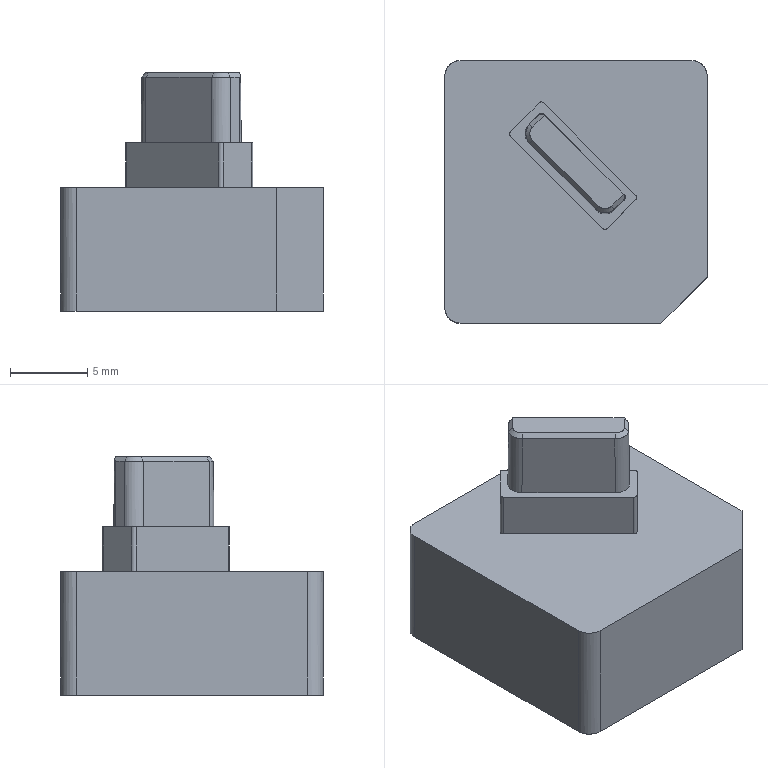NC program | PowerMill | posted with a generic post | part box 17 x 17 x 15.424 mm
Lines 2608 to 3246 of 24748:
N2705 M6
N2706 S8500 M03
N2707 G00 G90 X0.0 Y0.0
N2708 G43 Z11.804 H3
N2709
N2710 G05 P10000 R8
N2711 X-8.1622 Y14.5705
N2712 Z-3.7092
N2713 G01 Z-4.9092 F360.0
N2714 X-5.2505 Y10.1719 F600.0
N2715 X-4.7795 Y9.7047
N2716 G03 X-5.672 Y9.1307 I3.0048 J-5.6526
N2717 G01 X-5.9261 Y8.9205
N2718 X-6.1665 Y8.6947
N2719 X-6.7532 Y8.1079
N2720 X-6.943 Y7.9079
N2721 G03 X-7.4693 Y7.2473 I6.5097 J-5.7258
N2722 G01 X-7.6194 Y7.014
N2723 X-7.7808 Y6.7353
N2724 X-7.9298 Y6.4498
N2725 X-8.4896 Y7.0052
N2726 G00 Z5.8713
N2727 G01 X-8.3234 Y5.386 F10000.0
N2728 G00 Z-4.8092
N2729 G01 X-8.1838 Y5.8632 Z-4.8179 F360.0
N2730 X-8.0732 Y6.142 Z-4.8231
N2731 X-7.861 Y6.5856 Z-4.8317
N2732 X-7.6194 Y7.014 Z-4.8403
N2733 X-7.4693 Y7.2473 Z-4.8451
N2734 X-7.2142 Y7.584 Z-4.8525
N2735 X-6.943 Y7.9079 Z-4.8599
N2736 X-6.7692 Y8.0911 Z-4.8643
N2737 X-6.7532 Y8.1079 Z-4.8647
N2738 X-6.1665 Y8.6947 Z-4.8792
N2739 X-5.9261 Y8.9205 Z-4.8849
N2740 X-5.672 Y9.1307 Z-4.8907
N2741 X-5.2377 Y9.4362 Z-4.8999
N2742 X-4.7795 Y9.7047 Z-4.9092
N2743 X-4.408 Y9.8803 F600.0
N2744 X-4.0874 Y10.0038
N2745 X-3.7594 Y10.1061
N2746 G02 X-2.9536 Y10.2721 I1.8952 J-7.163
N2747 G01 X-2.5982 Y10.3085
N2748 X-2.2411 Y10.3207
N2749 X-1.884 Y10.3085
N2750 X-1.5285 Y10.2721
N2751 X-1.0566 Y10.1868
N2752 X-0.7227 Y10.1061
N2753 G02 X-0.0742 Y9.8803 I-1.5958 J-5.6266
N2754 G01 X0.2376 Y9.736
N2755 G02 X0.8297 Y9.388 I-2.6446 J-5.1761
N2756 G01 X1.1898 Y9.1307
N2757 X1.4429 Y8.9192
N2758 X1.6843 Y8.6947
N2759 X6.8169 Y3.5621
N2760 X7.0418 Y3.3209
N2761 X7.2529 Y3.0676
N2762 G02 X7.6939 Y2.4171 I-5.8869 J-4.466
N2763 G01 X7.8582 Y2.1154
N2764 X8.0025 Y1.8036
N2765 G02 X8.2429 Y1.0948 I-4.9188 J-2.0636
N2766 G01 X8.3338 Y0.7014
N2767 X8.3943 Y0.3493
N2768 G02 X8.4429 Y-0.3633 I-6.2851 J-0.7865
N2769 G01 X8.4307 Y-0.7204
N2770 X8.3943 Y-1.0759
N2771 X8.3338 Y-1.428
N2772 X8.2257 Y-1.8902
N2773 X8.126 Y-2.2096
N2774 G02 X7.8582 Y-2.842 I-5.4983 J1.9554
N2775 G01 X7.6939 Y-3.1437
N2776 X7.5102 Y-3.434
N2777 G02 X7.0427 Y-4.0483 I-5.0394 J3.3504
N2778 G01 X6.8169 Y-4.2887
N2779 X6.3459 Y-4.7598
N2780 G02 X5.5221 Y-5.4769 I-4.7037 J4.5714
N2781 G01 X5.3696 Y-5.5915
N2782 X5.0503 Y-5.797
N2783 G02 X4.2642 Y-6.1955 I-4.3291 J7.5645
N2784 G01 X3.9854 Y-6.3061
N2785 X3.7008 Y-6.4006
N2786 G02 X2.6002 Y-6.6355 I-2.1014 J7.1496
N2787 G01 X2.2932 Y-6.6626
N2788 X1.8786 Y-6.672
N2789 X1.464 Y-6.6626
N2790 X1.1571 Y-6.6355
N2791 X0.8523 Y-6.5904
N2792 G02 X-0.2282 Y-6.306 I1.3299 J7.2474
N2793 G01 X-0.507 Y-6.1955
N2794 G02 X-1.6123 Y-5.5915 I2.7732 J6.3884
N2795 G01 X-1.9159 Y-5.3635
N2796 G02 X-2.4729 Y-4.8755 I3.9536 J5.0749
N2797 G01 X-6.7532 Y-0.5952
N2798 G02 X-7.2412 Y-0.0381 I4.6108 J4.5318
N2799 G01 X-7.4692 Y0.2654
N2800 X-7.6747 Y0.5847
N2801 G02 X-8.0732 Y1.3708 I7.6482 J4.3716
N2802 G02 X-8.3564 Y2.2238 I5.0677 J2.1558
N2803 G02 X-8.5133 Y3.0348 I6.3457 J1.648
N2804 G01 X-8.5404 Y3.3418
N2805 G02 X-8.5133 Y4.4779 I7.4238 J0.3914
N2806 G02 X-8.1838 Y5.8632 I6.9185 J-0.9134
N2807 G01 X-8.0732 Y6.142
N2808 G02 X-7.6194 Y7.014 I6.7125 J-2.9395
N2809 G01 X-7.4693 Y7.2473
N2810 G02 X-6.943 Y7.9079 I7.036 J-5.0652
N2811 G01 X-6.7532 Y8.1079
N2812 X-6.1665 Y8.6947
N2813 X-5.9261 Y8.9205
N2814 X-5.672 Y9.1307
N2815 G02 X-4.7795 Y9.7047 I3.8973 J-5.0786
N2816 G00 Z4.0043
N2817 G01 X11.9477 Y-5.849 F10000.0
N2818 G00 Z0.8043
N2819 G01 Z-0.3957 F360.0
N2820 X7.4899 Y-3.0288 F600.0
N2821 X-4.7276 Y9.4739
N2822 X-4.9227 Y9.3603
N2823 X-5.3702 Y9.0347
N2824 X-5.4753 Y8.947
N2825 X-5.8176 Y8.6272
N2826 X-6.7123 Y7.7236
N2827 X-6.8167 Y7.605
N2828 X-7.1706 Y7.1572
N2829 X-7.4577 Y6.7094
N2830 X-7.5609 Y6.5138
N2831 X4.4533 Y-5.7809
N2832 G00 Z11.804
N2833 G05 P0
N2834 (---------------)
N2835 ( END TOOLPATH : 粗公基准台01-平坦面平行-D10 )
N2836 (---------------)
N2837 ( START TOOLPATH : 粗公基准台01-基准面偏置-D10 )
N2838 (---------------)
N2839 G00 X0.0 Y0.0 Z9.8043
N2840 G05 P10000 R8
N2841 X-2.368 Y19.035
N2842 Z-6.42
N2843 G01 Z-7.62 F360.0
N2844 X-2.3679 Y13.76 F600.0
N2845 X-2.3306 Y11.0677
N2846 G02 X-1.5285 Y11.0212 I0.0777 J-5.5932
N2847 G01 X-1.0969 Y10.9442
N2848 X-0.763 Y10.8635
N2849 X-0.435 Y10.7612
N2850 G02 X0.1974 Y10.4935 I-1.9637 J-5.5178
N2851 G01 X0.4991 Y10.3291
N2852 G02 X1.1182 Y9.9094 I-3.4177 J-5.708
N2853 G01 X1.3715 Y9.6983
N2854 X1.6127 Y9.4735
N2855 X7.5957 Y3.4904
N2856 X7.8214 Y3.25
N2857 G02 X8.6157 Y2.0751 I-4.4126 J-3.8388
N2858 G01 X8.7599 Y1.7633
N2859 X8.8835 Y1.4428
N2860 X8.9858 Y1.1148
N2861 X9.0664 Y0.7809
N2862 G02 X9.1798 Y-0.0062 I-5.9029 J-1.2522
N2863 G01 X9.192 Y-0.3633
N2864 X9.1798 Y-0.7204
N2865 X9.1434 Y-1.0758
N2866 X9.0659 Y-1.5095
N2867 X8.9858 Y-1.8414
N2868 X8.8835 Y-2.1694
N2869 X8.7599 Y-2.4899
N2870 X8.6157 Y-2.8017
N2871 X8.4513 Y-3.1034
N2872 X8.2255 Y-3.4557
N2873 X8.0317 Y-3.7225
N2874 X7.8215 Y-3.9766
N2875 X7.5957 Y-4.217
N2876 X5.7323 Y-6.0804
N2877 X5.4912 Y-6.3053
N2878 X5.2378 Y-6.5163
N2879 G02 X4.317 Y-7.1003 I-3.6863 J4.7942
N2880 G01 X4.0052 Y-7.2446
N2881 X3.6847 Y-7.3681
N2882 X3.3567 Y-7.4704
N2883 G02 X2.2357 Y-7.6645 I-1.6096 J5.9637
N2884 G02 X1.0756 Y-7.6125 I-0.3458 J5.2547
N2885 G01 X0.7345 Y-7.5511
N2886 G02 X-0.5822 Y-7.0882 I1.0963 J5.2223
N2887 G01 X-0.8615 Y-6.936
N2888 G02 X-1.4806 Y-6.5164 I3.4923 J5.8183
N2889 G01 X-1.7339 Y-6.3052
N2890 X-1.9751 Y-6.0804
N2891 X-3.5935 Y-4.462
N2892 X-6.991 Y-7.8595
N2893 G02 X-7.8827 Y-8.7514 I-0.4459 J-0.4459
N2894 G01 X-8.7516 Y-7.8829
N2895 G02 X-8.7517 Y-6.9908 I0.4459 J0.4461
N2896 G02 X-7.8596 I0.446 J-0.446
N2897 G01 X-6.991 Y-7.8595
N2898 X-3.5935 Y-4.462
N2899 X-7.9582 Y-0.0973
N2900 X-8.1829 Y0.144
N2901 X-8.3941 Y0.3971
N2902 X-8.6301 Y0.7259
N2903 X-8.8138 Y1.0163
N2904 X-8.9781 Y1.3179
N2905 X-9.1224 Y1.6298
N2906 X-9.2459 Y1.9503
N2907 G02 X-9.4453 Y2.6917 I5.5688 J1.8955
N2908 G01 X-9.5058 Y3.0438
N2909 X-9.5423 Y3.3993
N2910 X-9.5544 Y3.7564
N2911 X-9.5423 Y4.1135
N2912 X-9.5058 Y4.4689
N2913 X-9.4289 Y4.9005
N2914 X-9.3482 Y5.2345
N2915 X-9.2459 Y5.5624
N2916 G02 X-8.9781 Y6.1948 I5.5451 J-1.9752
N2917 G02 X-8.5484 Y6.9033 I4.9388 J-2.5112
N2918 G01 X-8.3941 Y7.1156
N2919 X-8.1839 Y7.3697
N2920 X-7.9582 Y7.6101
N2921 X-6.0948 Y9.4735
N2922 G02 X-5.2715 Y10.1454 I3.9028 J-3.9416
N2923 G01 X-4.9812 Y10.3291
N2924 X-4.6795 Y10.4935
N2925 X-4.3677 Y10.6377
N2926 X-4.0467 Y10.76
N2927 X-3.7192 Y10.8636
N2928 G02 X-2.9536 Y11.0211 I1.7771 J-6.6944
N2929 G01 X-2.5982 Y11.0576
N2930 X-2.3306 Y11.0677
N2931 X-2.3679 Y13.76
N2932 G00 Z9.8043
N2933 G05 P0
N2934 (---------------)
N2935 ( END TOOLPATH : 粗公基准台01-基准面偏置-D10 )
N2936 (---------------)
N2937 ( START TOOLPATH : 粗公基准台01-外形侧光-D10 )
N2938 (---------------)
N2939 G00 X0.0 Y0.0 Z10.804
N2940 G05 P10000 R8
N2941 X7.47 Y-4.439
N2942 Z-6.39
N2943 G01 Z-7.59 F360.0
N2944 G03 X6.4095 Y-4.8787 I0.0005 J-1.5 F600.0
N2945 G01 X5.4224 Y-5.8664
N2946 G02 X-1.6666 Y-5.865 I-3.5438 J3.6493
N2947 G01 X-4.6693 Y-2.8626
N2948 X-7.6732 Y0.141
N2949 G02 X-7.6721 Y7.373 I3.5784 J3.6154
N2950 G01 X-6.8152 Y8.2298
N2951 X-5.8221 Y9.2228
N2952 G02 X1.3419 Y9.221 I3.5811 J-3.6118
N2953 G01 X7.2798 Y3.2831
N2954 G02 X7.4142 Y-3.8733 I-3.5486 J-3.6461
N2955 G01 X6.4095 Y-4.8787
N2956 G03 X5.9705 Y-5.9395 I1.061 J-1.0603
N2957 G01 X7.4133 Y-4.3825
N2958 G03 X6.3528 Y-4.8222 I0.0005 J-1.5
N2959 G01 X5.3673 Y-5.8084
N2960 G02 X-1.6101 I-3.4887 J3.5911
N2961 G01 X-4.6128 Y-2.806
N2962 X-7.6155 Y0.1964
N2963 G02 Y7.3164 I3.5206 J3.56
N2964 G01 X-6.7586 Y8.1732
N2965 X-5.7675 Y9.1644
N2966 G02 X1.2853 I3.5264 J-3.5534
N2967 G01 X7.3573 Y3.0905
N2968 G02 Y-3.8171 I-3.6245 J-3.4538
N2969 G01 X6.3528 Y-4.8222
N2970 G03 X5.9138 Y-5.883 I1.061 J-1.0603
N2971 G00 Z10.804
N2972 G05 P0
N2973 (---------------)
N2974 ( END TOOLPATH : 粗公基准台01-外形侧光-D10 )
N2975 (---------------)
N2976 ( START TOOLPATH : 粗公基准台01-基准台侧光-D10 )
N2977 (---------------)
N2978 G00 X0.0 Y0.0 Z9.8043
N2979 G05 P10000 R8
N2980 X13.4843 Y-14.7706
N2981 Z-14.32
N2982 G01 Z-15.52 F360.0
N2983 G03 X9.9488 Y-11.2351 I-1.7677 J1.7677 F600.0
N2984 G01 X9.0587 Y-12.1252
N2985 X9.0582 Y-12.1257
N2986 X9.0577 Y-12.1262
N2987 X8.9953 Y-12.1864
N2988 X8.9933 Y-12.1883
N2989 X8.9913 Y-12.19
N2990 X8.5443 Y-12.5666
N2991 X8.5408 Y-12.5694
N2992 X8.5371 Y-12.572
N2993 X8.0901 Y-12.87
N2994 X8.0872 Y-12.8719
N2995 X8.0842 Y-12.8736
N2996 X7.7935 Y-13.0328
N2997 X7.7918 Y-13.0337
N2998 X7.79 Y-13.0346
N2999 X7.6336 Y-13.1102
N3000 X7.6312 Y-13.1114
N3001 X7.6288 Y-13.1124
N3002 X7.1818 Y-13.2935
N3003 X7.1783 Y-13.2948
N3004 X7.1746 Y-13.296
N3005 X6.7277 Y-13.4293
N3006 X6.7248 Y-13.4301
N3007 X6.722 Y-13.4308
N3008 X6.4639 Y-13.4877
N3009 X6.4621 Y-13.4881
N3010 X6.4603 Y-13.4884
N3011 X6.2714 Y-13.5211
N3012 X6.2689 Y-13.5215
N3013 X6.2664 Y-13.5218
N3014 X5.8194 Y-13.5699
N3015 X5.816 Y-13.5702
N3016 X5.8125 Y-13.5704
N3017 X5.3656 Y-13.58
N3018 X5.3647
N3019 X5.3638
N3020 X-7.5988 Y-13.5791
N3021 X-7.6011 Y-13.579
N3022 X-7.6033 Y-13.5789
N3023 X-8.0503 Y-13.5532
N3024 X-8.053 Y-13.553
N3025 X-8.0557 Y-13.5527
N3026 X-8.5027 Y-13.4965
N3027 X-8.5059 Y-13.496
N3028 X-8.5091 Y-13.4954
N3029 X-8.9561 Y-13.4017
N3030 X-8.9589 Y-13.4011
N3031 X-8.9617 Y-13.4003
N3032 X-9.4087 Y-13.2723
N3033 X-9.4118 Y-13.2713
N3034 X-9.4148 Y-13.2703
N3035 X-9.8618 Y-13.1025
N3036 X-9.8649 Y-13.1013
N3037 X-9.8679 Y-13.0999
N3038 X-10.3149 Y-12.8887
N3039 X-10.3178 Y-12.8872
N3040 X-10.3208 Y-12.8856
N3041 X-10.7677 Y-12.6268
N3042 X-10.7708 Y-12.6249
N3043 X-10.7738 Y-12.6229
N3044 X-11.2208 Y-12.3073
N3045 X-11.2238 Y-12.3051
N3046 X-11.2266 Y-12.3027
N3047 X-11.6736 Y-11.9205
N3048 X-11.676 Y-11.9184
N3049 X-11.6782 Y-11.9163
N3050 X-11.9163 Y-11.6782
N3051 X-11.9184 Y-11.676
N3052 X-11.9205 Y-11.6736
N3053 X-12.3027 Y-11.2266
N3054 X-12.3049 Y-11.224
N3055 X-12.307 Y-11.2213
N3056 X-12.5806 Y-10.8396
N3057 X-12.5827 Y-10.8365
N3058 X-12.5846 Y-10.8334
N3059 X-12.8853 Y-10.3212
N3060 X-12.8871 Y-10.318
N3061 X-12.8887 Y-10.3149
N3062 X-13.0999 Y-9.8679
N3063 X-13.1013 Y-9.8649
N3064 X-13.1025 Y-9.8618
N3065 X-13.2703 Y-9.4148
N3066 X-13.2713 Y-9.4118
N3067 X-13.2723 Y-9.4087
N3068 X-13.4003 Y-8.9617
N3069 X-13.4011 Y-8.9591
N3070 X-13.4017 Y-8.9564
N3071 X-13.4878 Y-8.5527
N3072 X-13.4884 Y-8.5495
N3073 X-13.4889 Y-8.5463
N3074 X-13.5527 Y-8.0561
N3075 X-13.553 Y-8.0532
N3076 X-13.5532 Y-8.0503
N3077 X-13.5789 Y-7.6033
N3078 X-13.579 Y-7.6011
N3079 X-13.5791 Y-7.5988
N3080 Y7.5988
N3081 X-13.579 Y7.6011
N3082 X-13.5789 Y7.6033
N3083 X-13.5532 Y8.0503
N3084 X-13.553 Y8.053
N3085 X-13.5527 Y8.0557
N3086 X-13.4965 Y8.5027
N3087 X-13.496 Y8.5059
N3088 X-13.4954 Y8.5091
N3089 X-13.4017 Y8.9561
N3090 X-13.4011 Y8.9589
N3091 X-13.4003 Y8.9617
N3092 X-13.2723 Y9.4087
N3093 X-13.2713 Y9.4118
N3094 X-13.2703 Y9.4148
N3095 X-13.1025 Y9.8618
N3096 X-13.1013 Y9.8649
N3097 X-13.0999 Y9.8679
N3098 X-12.8887 Y10.3149
N3099 X-12.8872 Y10.3178
N3100 X-12.8856 Y10.3208
N3101 X-12.6268 Y10.7677
N3102 X-12.6249 Y10.7708
N3103 X-12.6229 Y10.7738
N3104 X-12.3073 Y11.2208
N3105 X-12.3051 Y11.2238
N3106 X-12.3027 Y11.2266
N3107 X-11.9205 Y11.6736
N3108 X-11.9184 Y11.676
N3109 X-11.9163 Y11.6782
N3110 X-11.6782 Y11.9163
N3111 X-11.676 Y11.9184
N3112 X-11.6736 Y11.9205
N3113 X-11.2266 Y12.3027
N3114 X-11.224 Y12.3049
N3115 X-11.2213 Y12.307
N3116 X-10.8396 Y12.5806
N3117 X-10.8365 Y12.5827
N3118 X-10.8334 Y12.5846
N3119 X-10.3212 Y12.8853
N3120 X-10.318 Y12.8871
N3121 X-10.3149 Y12.8887
N3122 X-9.8679 Y13.0999
N3123 X-9.8649 Y13.1013
N3124 X-9.8618 Y13.1025
N3125 X-9.4148 Y13.2703
N3126 X-9.4118 Y13.2713
N3127 X-9.4087 Y13.2723
N3128 X-8.9617 Y13.4003
N3129 X-8.9591 Y13.4011
N3130 X-8.9564 Y13.4017
N3131 X-8.5527 Y13.4878
N3132 X-8.5495 Y13.4884
N3133 X-8.5463 Y13.4889
N3134 X-8.0561 Y13.5527
N3135 X-8.0532 Y13.553
N3136 X-8.0503 Y13.5532
N3137 X-7.6033 Y13.5789
N3138 X-7.6011 Y13.579
N3139 X-7.5988 Y13.5791
N3140 X0.0
N3141 X7.5988
N3142 X7.601 Y13.579
N3143 X7.6033 Y13.5789
N3144 X8.0503 Y13.5533
N3145 X8.053 Y13.5531
N3146 X8.0557 Y13.5528
N3147 X8.5027 Y13.4965
N3148 X8.5059 Y13.496
N3149 X8.5091 Y13.4954
N3150 X8.9561 Y13.4017
N3151 X8.9589 Y13.4011
N3152 X8.9617 Y13.4003
N3153 X9.4087 Y13.2723
N3154 X9.4118 Y13.2713
N3155 X9.4148 Y13.2703
N3156 X9.8618 Y13.1025
N3157 X9.8649 Y13.1013
N3158 X9.8679 Y13.0999
N3159 X10.3149 Y12.8887
N3160 X10.3178 Y12.8872
N3161 X10.3208 Y12.8856
N3162 X10.7677 Y12.6268
N3163 X10.7708 Y12.6249
N3164 X10.7738 Y12.6229
N3165 X11.2208 Y12.3073
N3166 X11.2238 Y12.3051
N3167 X11.2266 Y12.3027
N3168 X11.6736 Y11.9205
N3169 X11.676 Y11.9184
N3170 X11.6782 Y11.9163
N3171 X11.9163 Y11.6782
N3172 X11.9184 Y11.676
N3173 X11.9205 Y11.6736
N3174 X12.3027 Y11.2266
N3175 X12.3049 Y11.224
N3176 X12.307 Y11.2213
N3177 X12.5806 Y10.8396
N3178 X12.5827 Y10.8365
N3179 X12.5846 Y10.8334
N3180 X12.8853 Y10.3212
N3181 X12.8871 Y10.318
N3182 X12.8887 Y10.3149
N3183 X13.0999 Y9.8679
N3184 X13.1013 Y9.8649
N3185 X13.1025 Y9.8618
N3186 X13.2703 Y9.4148
N3187 X13.2713 Y9.4118
N3188 X13.2723 Y9.4087
N3189 X13.4003 Y8.9617
N3190 X13.401 Y8.9591
N3191 X13.4016 Y8.9564
N3192 X13.4878 Y8.5527
N3193 X13.4884 Y8.5495
N3194 X13.4889 Y8.5463
N3195 X13.5527 Y8.0561
N3196 X13.553 Y8.0532
N3197 X13.5532 Y8.0503
N3198 X13.5789 Y7.6033
N3199 X13.579 Y7.6011
N3200 X13.5791 Y7.5988
N3201 X13.58 Y-5.3638
N3202 Y-5.3647
N3203 Y-5.3656
N3204 X13.5704 Y-5.8125
N3205 X13.5702 Y-5.816
N3206 X13.5699 Y-5.8194
N3207 X13.5218 Y-6.2664
N3208 X13.5215 Y-6.2689
N3209 X13.5211 Y-6.2715
N3210 X13.4884 Y-6.4603
N3211 X13.4881 Y-6.4621
N3212 X13.4877 Y-6.4639
N3213 X13.4308 Y-6.722
N3214 X13.4301 Y-6.7248
N3215 X13.4293 Y-6.7277
N3216 X13.296 Y-7.1746
N3217 X13.2948 Y-7.1783
N3218 X13.2935 Y-7.1818
N3219 X13.1124 Y-7.6288
N3220 X13.1114 Y-7.6312
N3221 X13.1102 Y-7.6336
N3222 X13.0346 Y-7.79
N3223 X13.0337 Y-7.7918
N3224 X13.0328 Y-7.7935
N3225 X12.8736 Y-8.0842
N3226 X12.8719 Y-8.0871
N3227 X12.8701 Y-8.09
N3228 X12.5822 Y-8.5234
N3229 X12.5797 Y-8.527
N3230 X12.5769 Y-8.5305
N3231 X12.1901 Y-8.9912
N3232 X12.1883 Y-8.9932
N3233 X12.1864 Y-8.9953
N3234 X12.1262 Y-9.0577
N3235 X12.1257 Y-9.0582
N3236 X12.1252 Y-9.0587
N3237 X9.9488 Y-11.2351
N3238 G03 X13.4843 Y-14.7706 I1.7678 J-1.7678
N3239 G01 X13.433 Y-14.7089
N3240 G03 X9.8974 Y-11.1733 I-1.7678 J1.7678
N3241 G01 X9.0022 Y-12.0686
N3242 X8.9397 Y-12.1289
N3243 X8.4927 Y-12.5055
N3244 X8.0457 Y-12.8034
N3245 X7.7551 Y-12.9626
N3246 X7.5988 Y-13.0382
N3247 X7.1518 Y-13.2193
N3248 X6.7048 Y-13.3527
N3249 X6.4467 Y-13.4096
N3250 X6.2578 Y-13.4422
N3251 X5.8108 Y-13.4904
N3252 X5.3638 Y-13.5
N3253 X-7.5988 Y-13.4991
N3254 X-8.0457 Y-13.4734
N3255 X-8.4927 Y-13.4171
N3256 X-8.9397 Y-13.3234
N3257 X-9.3867 Y-13.1954
N3258 X-9.8337 Y-13.0276
N3259 X-10.2807 Y-12.8163
N3260 X-10.7277 Y-12.5576
N3261 X-11.1746 Y-12.2419
N3262 X-11.6216 Y-11.8597
N3263 X-11.8597 Y-11.6216
N3264 X-12.2419 Y-11.1746
N3265 X-12.5156 Y-10.7929
N3266 X-12.8163 Y-10.2807
N3267 X-13.0276 Y-9.8337
N3268 X-13.1954 Y-9.3867
N3269 X-13.3234 Y-8.9397
N3270 X-13.4096 Y-8.536
N3271 X-13.4734 Y-8.0457
N3272 X-13.4991 Y-7.5988
N3273 Y7.5988
N3274 X-13.4734 Y8.0457
N3275 X-13.4171 Y8.4927
N3276 X-13.3234 Y8.9397
N3277 X-13.1954 Y9.3867
N3278 X-13.0276 Y9.8337
N3279 X-12.8163 Y10.2807
N3280 X-12.5576 Y10.7277
N3281 X-12.2419 Y11.1746
N3282 X-11.8597 Y11.6216
N3283 X-11.6216 Y11.8597
N3284 X-11.1746 Y12.2419
N3285 X-10.7929 Y12.5156
N3286 X-10.2807 Y12.8163
N3287 X-9.8337 Y13.0276
N3288 X-9.3867 Y13.1954
N3289 X-8.9397 Y13.3234
N3290 X-8.536 Y13.4096
N3291 X-8.0457 Y13.4734
N3292 X-7.5988 Y13.4991
N3293 X0.0
N3294 X7.5988
N3295 X8.0457 Y13.4734
N3296 X8.4927 Y13.4171
N3297 X8.9397 Y13.3234
N3298 X9.3867 Y13.1954
N3299 X9.8337 Y13.0276
N3300 X10.2807 Y12.8163
N3301 X10.7277 Y12.5576
N3302 X11.1746 Y12.2419
N3303 X11.6216 Y11.8597
N3304 X11.8597 Y11.6216
N3305 X12.2419 Y11.1746
N3306 X12.5156 Y10.7929
N3307 X12.8163 Y10.2807
N3308 X13.0276 Y9.8337
N3309 X13.1954 Y9.3867
N3310 X13.3234 Y8.9397
N3311 X13.4096 Y8.536
N3312 X13.4734 Y8.0457
N3313 X13.4991 Y7.5988
N3314 X13.5 Y-5.3638
N3315 X13.4904 Y-5.8108
N3316 X13.4423 Y-6.2578
N3317 X13.4096 Y-6.4467
N3318 X13.3527 Y-6.7048
N3319 X13.2193 Y-7.1518
N3320 X13.0382 Y-7.5988
N3321 X12.9626 Y-7.7551
N3322 X12.8034 Y-8.0457
N3323 X12.5156 Y-8.4791
N3324 X12.1289 Y-8.9397
N3325 X12.0686 Y-9.0022
N3326 X9.8974 Y-11.1733
N3327 G03 X13.433 Y-14.7089 I1.7678 J-1.7678
N3328 G00 Z9.8043
N3329 G05 P0
N3330 (---------------)
N3331 ( END TOOLPATH : 粗公基准台01-基准台侧光-D10 )
N3332 (---------------)
N3333
N3334 M05
N3335 G53 Z0.0
N3336 (---------------)
N3337 ( START TOOLPATH : 粗公精光01-等高-D4 )
N3338 (---------------)
N3339 ( TOOL NO.    :14 )
N3340 ( TOOL TYPE   : ENDMILL)
N3341 ( TOOL ID     : D4_2_1)
N3342 ( TOOL DIA    : 4.0 LENGTH 62.44)
N3343 T14